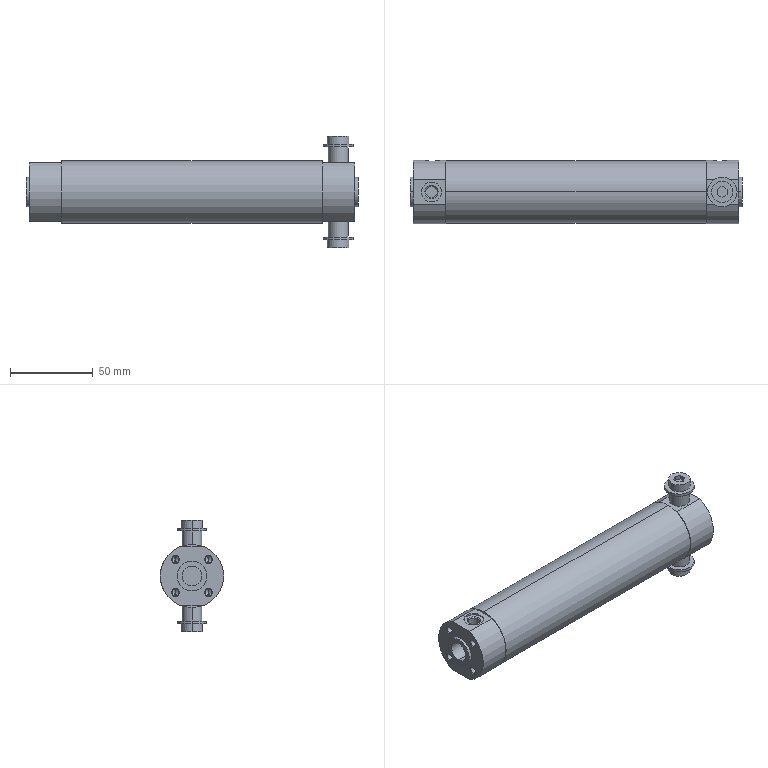Part | SolidWorks | features BaseBody 1 | 1 solid | 140 faces | box 201 x 38.4 x 67.7 mm | volume 158139 mm3 | cylinder 54 | cone 44 | plane 42 | commonest cylinder face diameters 4.134 x16 12 x10 18 x8 6.917 x4 8.566 x4 13 x4